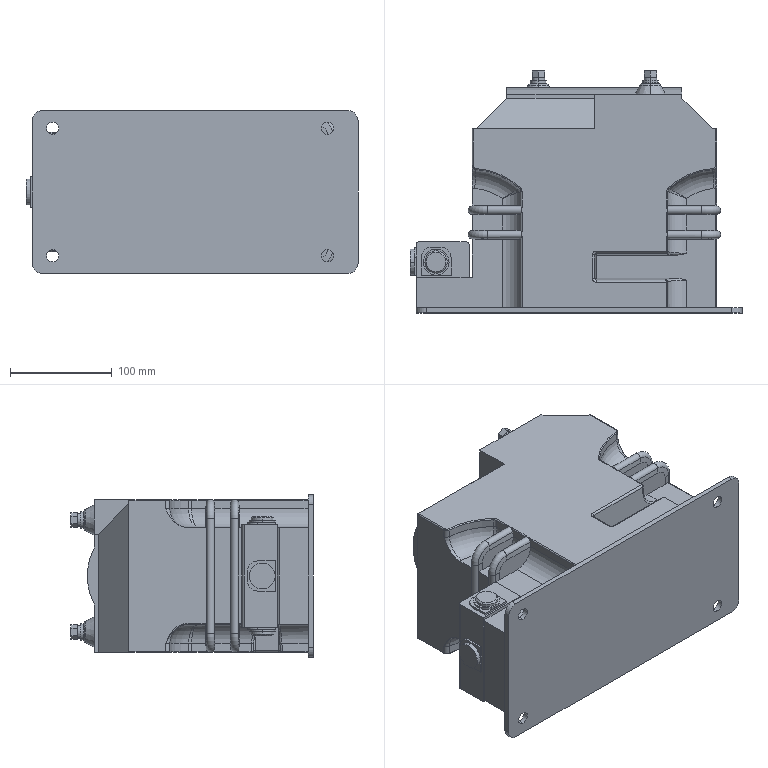Part | STEP file | JDZJ(X)10-10(R)(L) series voltage transformer(1).step | 2 solids | 369 faces | box 326.1 x 237.96 x 160 mm | volume 7233561 mm3 | plane 151 | cylinder 119 | torus 36 | spline 35 | cone 28 | commonest cylinder face diameters 2 x27 8 x20 37 x14 4 x11 12 x10 20 x10